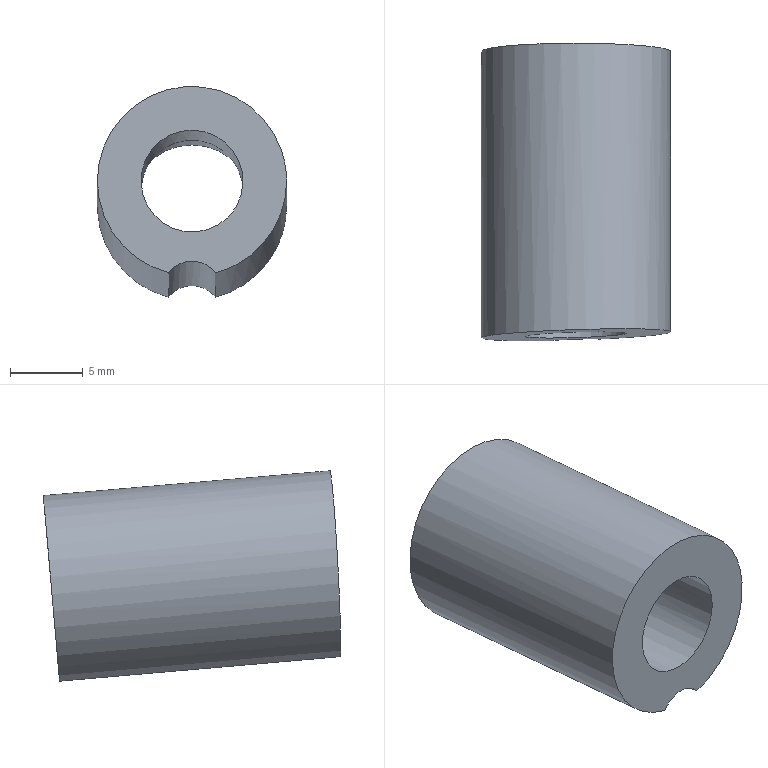Part | NX | features EKSD 13-20-7.000 2 | 1 solid | 9 faces | box 13 x 20.42 x 14.472 mm | volume 1595 mm3 | cylinder 6 | plane 3 | commonest cylinder face diameters 13 x2 4 x1 7 x1 8.4 x1 16 x1
STEP:
#1=CARTESIAN_POINT('',(-236.337,-57.903,-32.664));
#2=VERTEX_POINT('',#1);
#3=CARTESIAN_POINT('',(-236.337,-38.659,-34.348));
#4=VERTEX_POINT('',#3);
#5=CARTESIAN_POINT('',(-236.337,-48.362,-33.499));
#6=DIRECTION('',(0.,0.9962,-0.08716));
#7=VECTOR('',#6,1000.);
#8=LINE('',#5,#7);
#9=EDGE_CURVE('',#2,#4,#8,.T.);
#10=ORIENTED_EDGE('',*,*,#9,.F.);
#11=CARTESIAN_POINT('',(-241.235,-58.405,-39.104));
#12=VERTEX_POINT('',#11);
#13=CARTESIAN_POINT('',(-242.835,-58.122,-32.805));
#14=DIRECTION('',(-0.03252,0.9981,-0.05307));
#15=DIRECTION('',(0.6892,-0.01607,-0.7244));
#16=AXIS2_PLACEMENT_3D('',#13,#14,#15);
#17=ELLIPSE('',#16,6.507,6.5);
#18=EDGE_CURVE('',#2,#12,#17,.T.);
#19=ORIENTED_EDGE('',*,*,#18,.T.);
#20=CARTESIAN_POINT('',(-241.235,-39.222,-40.782));
#21=VERTEX_POINT('',#20);
#22=CARTESIAN_POINT('',(-241.235,-49.107,-39.917));
#23=DIRECTION('',(0.,0.9962,-0.08716));
#24=VECTOR('',#23,1000.);
#25=LINE('',#22,#24);
#26=EDGE_CURVE('',#21,#12,#25,.F.);
#27=ORIENTED_EDGE('',*,*,#26,.F.);
#28=CARTESIAN_POINT('',(-242.835,-38.673,-34.506));
#29=DIRECTION('',(0.,-0.9962,0.08716));
#30=DIRECTION('',(0.,-0.08716,-0.9962));
#31=AXIS2_PLACEMENT_3D('',#28,#29,#30);
#32=CIRCLE('',#31,6.5);
#33=EDGE_CURVE('',#21,#4,#32,.T.);
#34=ORIENTED_EDGE('',*,*,#33,.T.);
#35=EDGE_LOOP('',(#10,#19,#27,#34));
#36=FACE_BOUND('',#35,.T.);
#37=CARTESIAN_POINT('',(-242.835,-58.52,-32.77));
#38=DIRECTION('',(0.,0.9962,-0.08716));
#39=DIRECTION('',(1.,0.,0.));
#40=AXIS2_PLACEMENT_3D('',#37,#38,#39);
#41=CYLINDRICAL_SURFACE('',#40,6.5);
#42=ADVANCED_FACE('',(#36),#41,.T.);
#43=CARTESIAN_POINT('',(-236.363,-38.621,-33.91));
#44=VERTEX_POINT('',#43);
#45=CARTESIAN_POINT('',(-228.366,-38.599,-33.665));
#46=DIRECTION('',(0.,-0.9962,0.08716));
#47=DIRECTION('',(0.,-0.08716,-0.9962));
#48=AXIS2_PLACEMENT_3D('',#45,#46,#47);
#49=CIRCLE('',#48,8.);
#50=EDGE_CURVE('',#44,#4,#49,.T.);
#51=ORIENTED_EDGE('',*,*,#50,.T.);
#52=ORIENTED_EDGE('',*,*,#33,.F.);
#53=CARTESIAN_POINT('',(-244.435,-39.222,-40.782));
#54=VERTEX_POINT('',#53);
#55=CARTESIAN_POINT('',(-242.835,-39.326,-41.978));
#56=DIRECTION('',(0.,-0.9962,0.08716));
#57=DIRECTION('',(0.,-0.08716,-0.9962));
#58=AXIS2_PLACEMENT_3D('',#55,#56,#57);
#59=CIRCLE('',#58,2.);
#60=EDGE_CURVE('',#21,#54,#59,.T.);
#61=ORIENTED_EDGE('',*,*,#60,.T.);
#62=CARTESIAN_POINT('',(-242.835,-38.673,-34.506));
#63=DIRECTION('',(0.,-0.9962,0.08716));
#64=DIRECTION('',(0.,-0.08716,-0.9962));
#65=AXIS2_PLACEMENT_3D('',#62,#63,#64);
#66=CIRCLE('',#65,6.5);
#67=EDGE_CURVE('',#44,#54,#66,.T.);
#68=ORIENTED_EDGE('',*,*,#67,.F.);
#69=EDGE_LOOP('',(#51,#52,#61,#68));
#70=FACE_BOUND('',#69,.T.);
#71=CARTESIAN_POINT('',(-242.835,-39.039,-38.69));
#72=VERTEX_POINT('',#71);
#73=CARTESIAN_POINT('',(-242.835,-38.673,-34.506));
#74=DIRECTION('',(0.,-0.9962,0.08716));
#75=DIRECTION('',(0.,-0.08716,-0.9962));
#76=AXIS2_PLACEMENT_3D('',#73,#74,#75);
#77=CIRCLE('',#76,4.2);
#78=EDGE_CURVE('',#72,#72,#77,.F.);
#79=ORIENTED_EDGE('',*,*,#78,.F.);
#80=EDGE_LOOP('',(#79));
#81=FACE_BOUND('',#80,.T.);
#82=CARTESIAN_POINT('',(-228.366,-38.62,-33.907));
#83=DIRECTION('',(0.,-0.9962,0.08716));
#84=DIRECTION('',(0.,-0.08716,-0.9962));
#85=AXIS2_PLACEMENT_3D('',#82,#83,#84);
#86=PLANE('',#85);
#87=ADVANCED_FACE('',(#70,#81),#86,.F.);
#88=CARTESIAN_POINT('',(-236.363,-57.88,-32.225));
#89=VERTEX_POINT('',#88);
#90=CARTESIAN_POINT('',(-228.366,-57.608,-32.002));
#91=DIRECTION('',(-0.03252,0.9981,-0.05307));
#92=DIRECTION('',(0.6892,-0.01607,-0.7244));
#93=AXIS2_PLACEMENT_3D('',#90,#91,#92);
#94=ELLIPSE('',#93,8.009,8.);
#95=EDGE_CURVE('',#89,#2,#94,.F.);
#96=ORIENTED_EDGE('',*,*,#95,.F.);
#97=CARTESIAN_POINT('',(-244.435,-58.508,-39.095));
#98=VERTEX_POINT('',#97);
#99=CARTESIAN_POINT('',(-242.835,-58.122,-32.805));
#100=DIRECTION('',(-0.03252,0.9981,-0.05307));
#101=DIRECTION('',(0.6892,-0.01607,-0.7244));
#102=AXIS2_PLACEMENT_3D('',#99,#100,#101);
#103=ELLIPSE('',#102,6.507,6.5);
#104=EDGE_CURVE('',#98,#89,#103,.T.);
#105=ORIENTED_EDGE('',*,*,#104,.F.);
#106=CARTESIAN_POINT('',(-242.835,-58.52,-40.299));
#107=DIRECTION('',(-0.03252,0.9981,-0.05307));
#108=DIRECTION('',(0.6892,-0.01607,-0.7244));
#109=AXIS2_PLACEMENT_3D('',#106,#107,#108);
#110=ELLIPSE('',#109,2.002,2.);
#111=EDGE_CURVE('',#98,#12,#110,.T.);
#112=ORIENTED_EDGE('',*,*,#111,.T.);
#113=ORIENTED_EDGE('',*,*,#18,.F.);
#114=EDGE_LOOP('',(#96,#105,#112,#113));
#115=FACE_BOUND('',#114,.T.);
#116=CARTESIAN_POINT('',(-240.42,-58.178,-35.343));
#117=VERTEX_POINT('',#116);
#118=CARTESIAN_POINT('',(-242.835,-58.122,-32.805));
#119=DIRECTION('',(-0.03252,0.9981,-0.05307));
#120=DIRECTION('',(0.6892,-0.01607,-0.7244));
#121=AXIS2_PLACEMENT_3D('',#118,#119,#120);
#122=ELLIPSE('',#121,3.504,3.5);
#123=EDGE_CURVE('',#117,#117,#122,.F.);
#124=ORIENTED_EDGE('',*,*,#123,.F.);
#125=EDGE_LOOP('',(#124));
#126=FACE_BOUND('',#125,.T.);
#127=CARTESIAN_POINT('',(-422.194,-57.948,80.353));
#128=DIRECTION('',(-0.03252,0.9981,-0.05307));
#129=DIRECTION('',(0.05223,-0.05133,-0.9973));
#130=AXIS2_PLACEMENT_3D('',#127,#128,#129);
#131=PLANE('',#130);
#132=ADVANCED_FACE('',(#115,#126),#131,.F.);
#133=CARTESIAN_POINT('',(-236.363,-48.324,-33.061));
#134=DIRECTION('',(0.,0.9962,-0.08716));
#135=VECTOR('',#134,1000.);
#136=LINE('',#133,#135);
#137=EDGE_CURVE('',#44,#89,#136,.F.);
#138=ORIENTED_EDGE('',*,*,#137,.F.);
#139=ORIENTED_EDGE('',*,*,#67,.T.);
#140=CARTESIAN_POINT('',(-244.435,-49.107,-39.917));
#141=DIRECTION('',(0.,0.9962,-0.08716));
#142=VECTOR('',#141,1000.);
#143=LINE('',#140,#142);
#144=EDGE_CURVE('',#98,#54,#143,.T.);
#145=ORIENTED_EDGE('',*,*,#144,.F.);
#146=ORIENTED_EDGE('',*,*,#104,.T.);
#147=EDGE_LOOP('',(#138,#139,#145,#146));
#148=FACE_BOUND('',#147,.T.);
#149=CARTESIAN_POINT('',(-242.835,-58.52,-32.77));
#150=DIRECTION('',(0.,0.9962,-0.08716));
#151=DIRECTION('',(1.,0.,0.));
#152=AXIS2_PLACEMENT_3D('',#149,#150,#151);
#153=CYLINDRICAL_SURFACE('',#152,6.5);
#154=ADVANCED_FACE('',(#148),#153,.T.);
#155=CARTESIAN_POINT('',(-246.335,-50.551,-33.467));
#156=VERTEX_POINT('',#155);
#157=CARTESIAN_POINT('',(-242.835,-50.551,-33.467));
#158=DIRECTION('',(0.,-0.9962,0.08716));
#159=DIRECTION('',(-1.,0.,0.));
#160=AXIS2_PLACEMENT_3D('',#157,#158,#159);
#161=CIRCLE('',#160,3.5);
#162=EDGE_CURVE('',#156,#156,#161,.F.);
#163=ORIENTED_EDGE('',*,*,#162,.T.);
#164=EDGE_LOOP('',(#163));
#165=FACE_BOUND('',#164,.T.);
#166=ORIENTED_EDGE('',*,*,#123,.T.);
#167=EDGE_LOOP('',(#166));
#168=FACE_BOUND('',#167,.T.);
#169=CARTESIAN_POINT('',(-242.835,-59.516,-32.683));
#170=DIRECTION('',(0.,0.9962,-0.08716));
#171=DIRECTION('',(1.,0.,0.));
#172=AXIS2_PLACEMENT_3D('',#169,#170,#171);
#173=CYLINDRICAL_SURFACE('',#172,3.5);
#174=ADVANCED_FACE('',(#165,#168),#173,.F.);
#175=CARTESIAN_POINT('',(-238.635,-50.551,-33.467));
#176=VERTEX_POINT('',#175);
#177=CARTESIAN_POINT('',(-242.835,-50.551,-33.467));
#178=DIRECTION('',(0.,0.9962,-0.08716));
#179=DIRECTION('',(1.,0.,0.));
#180=AXIS2_PLACEMENT_3D('',#177,#178,#179);
#181=CIRCLE('',#180,4.2);
#182=EDGE_CURVE('',#176,#176,#181,.T.);
#183=ORIENTED_EDGE('',*,*,#182,.T.);
#184=EDGE_LOOP('',(#183));
#185=FACE_BOUND('',#184,.T.);
#186=ORIENTED_EDGE('',*,*,#162,.F.);
#187=EDGE_LOOP('',(#186));
#188=FACE_BOUND('',#187,.T.);
#189=CARTESIAN_POINT('',(-242.835,-50.551,-33.467));
#190=DIRECTION('',(0.,-0.9962,0.08716));
#191=DIRECTION('',(-1.,0.,0.));
#192=AXIS2_PLACEMENT_3D('',#189,#190,#191);
#193=PLANE('',#192);
#194=ADVANCED_FACE('',(#185,#188),#193,.F.);
#195=ORIENTED_EDGE('',*,*,#78,.T.);
#196=EDGE_LOOP('',(#195));
#197=FACE_BOUND('',#196,.T.);
#198=ORIENTED_EDGE('',*,*,#182,.F.);
#199=EDGE_LOOP('',(#198));
#200=FACE_BOUND('',#199,.T.);
#201=CARTESIAN_POINT('',(-242.835,-50.551,-33.467));
#202=DIRECTION('',(0.,0.9962,-0.08716));
#203=DIRECTION('',(1.,0.,0.));
#204=AXIS2_PLACEMENT_3D('',#201,#202,#203);
#205=CYLINDRICAL_SURFACE('',#204,4.2);
#206=ADVANCED_FACE('',(#197,#200),#205,.F.);
#207=ORIENTED_EDGE('',*,*,#144,.T.);
#208=ORIENTED_EDGE('',*,*,#60,.F.);
#209=ORIENTED_EDGE('',*,*,#26,.T.);
#210=ORIENTED_EDGE('',*,*,#111,.F.);
#211=EDGE_LOOP('',(#207,#208,#209,#210));
#212=FACE_BOUND('',#211,.T.);
#213=CARTESIAN_POINT('',(-242.835,-59.174,-40.241));
#214=DIRECTION('',(0.,0.9962,-0.08716));
#215=DIRECTION('',(1.,0.,0.));
#216=AXIS2_PLACEMENT_3D('',#213,#214,#215);
#217=CYLINDRICAL_SURFACE('',#216,2.);
#218=ADVANCED_FACE('',(#212),#217,.F.);
#219=ORIENTED_EDGE('',*,*,#9,.T.);
#220=ORIENTED_EDGE('',*,*,#50,.F.);
#221=ORIENTED_EDGE('',*,*,#137,.T.);
#222=ORIENTED_EDGE('',*,*,#95,.T.);
#223=EDGE_LOOP('',(#219,#220,#221,#222));
#224=FACE_BOUND('',#223,.T.);
#225=CARTESIAN_POINT('',(-228.366,-58.006,-31.967));
#226=DIRECTION('',(0.,0.9962,-0.08716));
#227=DIRECTION('',(-0.9997,-0.001977,-0.0226));
#228=AXIS2_PLACEMENT_3D('',#225,#226,#227);
#229=CYLINDRICAL_SURFACE('',#228,8.);
#230=ADVANCED_FACE('',(#224),#229,.F.);
#231=CLOSED_SHELL('',(#42,#87,#132,#154,#174,#194,#206,#218,#230));
#232=MANIFOLD_SOLID_BREP('',#231);
#233=(LENGTH_UNIT()NAMED_UNIT(*)SI_UNIT(.MILLI.,.METRE.));
#234=UNCERTAINTY_MEASURE_WITH_UNIT(LENGTH_MEASURE(0.00001),#233,'','');
#235=(NAMED_UNIT(*)PLANE_ANGLE_UNIT()SI_UNIT($,.RADIAN.));
#236=(NAMED_UNIT(*)SI_UNIT($,.STERADIAN.)SOLID_ANGLE_UNIT());
#237=(GEOMETRIC_REPRESENTATION_CONTEXT(3)GLOBAL_UNCERTAINTY_ASSIGNED_CONTEXT((#234))GLOBAL_UNIT_ASSIGNED_CONTEXT((#233,#235,#236))REPRESENTATION_CONTEXT('',''));
#238=ADVANCED_BREP_SHAPE_REPRESENTATION('',(#232),#237);